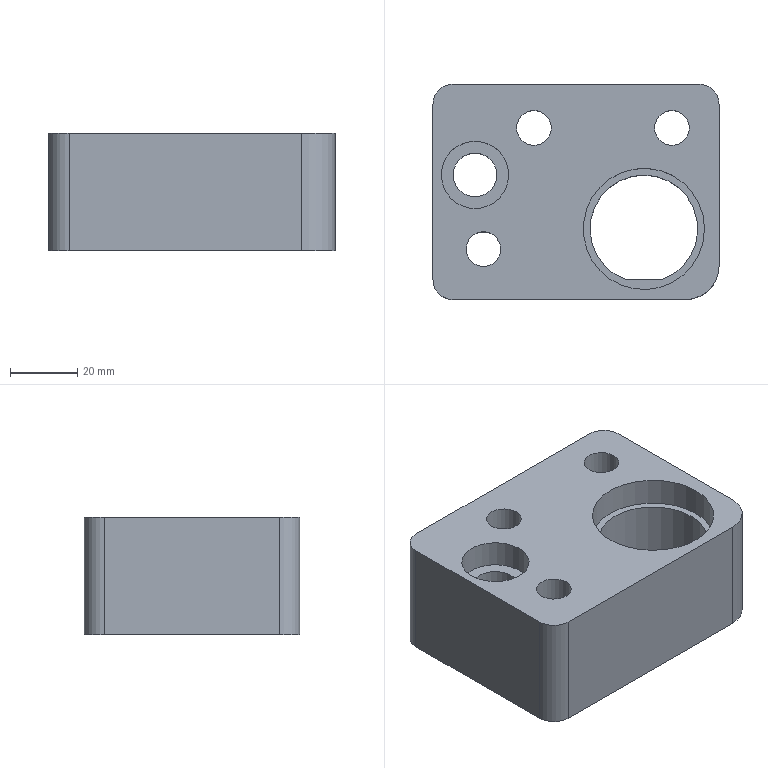Part | NX | features 7 2 | 1 solid | 26 faces | box 85 x 64 x 35 mm | volume 137595 mm3 | cylinder 14 | plane 12 | commonest cylinder face diameters 10.3 x3 12 x3 18 x3 20 x2 13 x1 32 x1
STEP:
#1=CARTESIAN_POINT('',(150.679,-398.,91.));
#2=VERTEX_POINT('',#1);
#3=CARTESIAN_POINT('',(145.529,-398.,91.));
#4=DIRECTION('',(0.,0.,-1.));
#5=DIRECTION('',(1.,0.,0.));
#6=AXIS2_PLACEMENT_3D('',#3,#4,#5);
#7=CIRCLE('',#6,5.15);
#8=EDGE_CURVE('',#2,#2,#7,.T.);
#9=ORIENTED_EDGE('',*,*,#8,.T.);
#10=EDGE_LOOP('',(#9));
#11=FACE_BOUND('',#10,.T.);
#12=CARTESIAN_POINT('',(97.029,-411.95,91.));
#13=VERTEX_POINT('',#12);
#14=CARTESIAN_POINT('',(87.029,-411.95,91.));
#15=DIRECTION('',(0.,0.,-1.));
#16=DIRECTION('',(1.,0.,0.));
#17=AXIS2_PLACEMENT_3D('',#14,#15,#16);
#18=CIRCLE('',#17,10.);
#19=EDGE_CURVE('',#13,#13,#18,.T.);
#20=ORIENTED_EDGE('',*,*,#19,.T.);
#21=EDGE_LOOP('',(#20));
#22=FACE_BOUND('',#21,.T.);
#23=CARTESIAN_POINT('',(155.199,-428.,91.));
#24=VERTEX_POINT('',#23);
#25=CARTESIAN_POINT('',(137.199,-428.,91.));
#26=DIRECTION('',(0.,0.,1.));
#27=DIRECTION('',(1.,0.,0.));
#28=AXIS2_PLACEMENT_3D('',#25,#26,#27);
#29=CIRCLE('',#28,18.);
#30=EDGE_CURVE('',#24,#24,#29,.T.);
#31=ORIENTED_EDGE('',*,*,#30,.F.);
#32=EDGE_LOOP('',(#31));
#33=FACE_BOUND('',#32,.T.);
#34=CARTESIAN_POINT('',(149.529,-449.,91.));
#35=VERTEX_POINT('',#34);
#36=CARTESIAN_POINT('',(80.529,-449.,91.));
#37=VERTEX_POINT('',#36);
#38=CARTESIAN_POINT('',(116.864,-449.,91.));
#39=DIRECTION('',(-1.,0.,0.));
#40=VECTOR('',#39,1000.);
#41=LINE('',#38,#40);
#42=EDGE_CURVE('',#35,#37,#41,.T.);
#43=ORIENTED_EDGE('',*,*,#42,.F.);
#44=CARTESIAN_POINT('',(159.529,-439.,91.));
#45=VERTEX_POINT('',#44);
#46=CARTESIAN_POINT('',(149.529,-439.,91.));
#47=DIRECTION('',(0.,0.,1.));
#48=DIRECTION('',(1.,0.,0.));
#49=AXIS2_PLACEMENT_3D('',#46,#47,#48);
#50=CIRCLE('',#49,10.);
#51=EDGE_CURVE('',#35,#45,#50,.T.);
#52=ORIENTED_EDGE('',*,*,#51,.T.);
#53=CARTESIAN_POINT('',(159.529,-391.,91.));
#54=VERTEX_POINT('',#53);
#55=CARTESIAN_POINT('',(159.529,-424.225,91.));
#56=DIRECTION('',(0.,-1.,0.));
#57=VECTOR('',#56,1000.);
#58=LINE('',#55,#57);
#59=EDGE_CURVE('',#54,#45,#58,.T.);
#60=ORIENTED_EDGE('',*,*,#59,.F.);
#61=CARTESIAN_POINT('',(153.529,-385.,91.));
#62=VERTEX_POINT('',#61);
#63=CARTESIAN_POINT('',(153.529,-391.,91.));
#64=DIRECTION('',(0.,0.,1.));
#65=DIRECTION('',(1.,0.,0.));
#66=AXIS2_PLACEMENT_3D('',#63,#64,#65);
#67=CIRCLE('',#66,6.);
#68=EDGE_CURVE('',#54,#62,#67,.T.);
#69=ORIENTED_EDGE('',*,*,#68,.T.);
#70=CARTESIAN_POINT('',(80.529,-385.,91.));
#71=VERTEX_POINT('',#70);
#72=CARTESIAN_POINT('',(116.864,-385.,91.));
#73=DIRECTION('',(1.,0.,0.));
#74=VECTOR('',#73,1000.);
#75=LINE('',#72,#74);
#76=EDGE_CURVE('',#71,#62,#75,.T.);
#77=ORIENTED_EDGE('',*,*,#76,.F.);
#78=CARTESIAN_POINT('',(74.529,-391.,91.));
#79=VERTEX_POINT('',#78);
#80=CARTESIAN_POINT('',(80.529,-391.,91.));
#81=DIRECTION('',(0.,0.,1.));
#82=DIRECTION('',(1.,0.,0.));
#83=AXIS2_PLACEMENT_3D('',#80,#81,#82);
#84=CIRCLE('',#83,6.);
#85=EDGE_CURVE('',#71,#79,#84,.T.);
#86=ORIENTED_EDGE('',*,*,#85,.T.);
#87=CARTESIAN_POINT('',(74.529,-443.,91.));
#88=VERTEX_POINT('',#87);
#89=CARTESIAN_POINT('',(74.529,-424.225,91.));
#90=DIRECTION('',(0.,1.,0.));
#91=VECTOR('',#90,1000.);
#92=LINE('',#89,#91);
#93=EDGE_CURVE('',#88,#79,#92,.T.);
#94=ORIENTED_EDGE('',*,*,#93,.F.);
#95=CARTESIAN_POINT('',(80.529,-443.,91.));
#96=DIRECTION('',(0.,0.,1.));
#97=DIRECTION('',(1.,0.,0.));
#98=AXIS2_PLACEMENT_3D('',#95,#96,#97);
#99=CIRCLE('',#98,6.);
#100=EDGE_CURVE('',#88,#37,#99,.T.);
#101=ORIENTED_EDGE('',*,*,#100,.T.);
#102=EDGE_LOOP('',(#43,#52,#60,#69,#77,#86,#94,#101));
#103=FACE_BOUND('',#102,.T.);
#104=CARTESIAN_POINT('',(109.679,-398.,91.));
#105=VERTEX_POINT('',#104);
#106=CARTESIAN_POINT('',(104.529,-398.,91.));
#107=DIRECTION('',(0.,0.,-1.));
#108=DIRECTION('',(1.,0.,0.));
#109=AXIS2_PLACEMENT_3D('',#106,#107,#108);
#110=CIRCLE('',#109,5.15);
#111=EDGE_CURVE('',#105,#105,#110,.T.);
#112=ORIENTED_EDGE('',*,*,#111,.T.);
#113=EDGE_LOOP('',(#112));
#114=FACE_BOUND('',#113,.T.);
#115=CARTESIAN_POINT('',(94.679,-434.,91.));
#116=VERTEX_POINT('',#115);
#117=CARTESIAN_POINT('',(89.529,-434.,91.));
#118=DIRECTION('',(0.,0.,-1.));
#119=DIRECTION('',(1.,0.,0.));
#120=AXIS2_PLACEMENT_3D('',#117,#118,#119);
#121=CIRCLE('',#120,5.15);
#122=EDGE_CURVE('',#116,#116,#121,.T.);
#123=ORIENTED_EDGE('',*,*,#122,.T.);
#124=EDGE_LOOP('',(#123));
#125=FACE_BOUND('',#124,.T.);
#126=CARTESIAN_POINT('',(87.029,-411.95,91.));
#127=DIRECTION('',(0.,0.,1.));
#128=DIRECTION('',(-1.,0.,0.));
#129=AXIS2_PLACEMENT_3D('',#126,#127,#128);
#130=PLANE('',#129);
#131=ADVANCED_FACE('',(#11,#22,#33,#103,#114,#125),#130,.T.);
#132=CARTESIAN_POINT('',(154.529,-398.,56.));
#133=VERTEX_POINT('',#132);
#134=CARTESIAN_POINT('',(145.529,-398.,56.));
#135=DIRECTION('',(0.,0.,1.));
#136=DIRECTION('',(1.,0.,0.));
#137=AXIS2_PLACEMENT_3D('',#134,#135,#136);
#138=CIRCLE('',#137,9.);
#139=EDGE_CURVE('',#133,#133,#138,.T.);
#140=ORIENTED_EDGE('',*,*,#139,.T.);
#141=EDGE_LOOP('',(#140));
#142=FACE_BOUND('',#141,.T.);
#143=CARTESIAN_POINT('',(80.529,-411.95,56.));
#144=VERTEX_POINT('',#143);
#145=CARTESIAN_POINT('',(87.029,-411.95,56.));
#146=DIRECTION('',(0.,0.,1.));
#147=DIRECTION('',(-1.,0.,0.));
#148=AXIS2_PLACEMENT_3D('',#145,#146,#147);
#149=CIRCLE('',#148,6.5);
#150=EDGE_CURVE('',#144,#144,#149,.T.);
#151=ORIENTED_EDGE('',*,*,#150,.T.);
#152=EDGE_LOOP('',(#151));
#153=FACE_BOUND('',#152,.T.);
#154=CARTESIAN_POINT('',(142.767,-443.,56.));
#155=VERTEX_POINT('',#154);
#156=CARTESIAN_POINT('',(131.631,-443.,56.));
#157=VERTEX_POINT('',#156);
#158=CARTESIAN_POINT('',(-89.971,-443.,56.));
#159=DIRECTION('',(-1.,0.,0.));
#160=VECTOR('',#159,1000.);
#161=LINE('',#158,#160);
#162=EDGE_CURVE('',#155,#157,#161,.T.);
#163=ORIENTED_EDGE('',*,*,#162,.F.);
#164=CARTESIAN_POINT('',(137.199,-428.,56.));
#165=DIRECTION('',(0.,0.,1.));
#166=DIRECTION('',(-1.,0.,0.));
#167=AXIS2_PLACEMENT_3D('',#164,#165,#166);
#168=CIRCLE('',#167,16.);
#169=EDGE_CURVE('',#155,#157,#168,.T.);
#170=ORIENTED_EDGE('',*,*,#169,.T.);
#171=EDGE_LOOP('',(#163,#170));
#172=FACE_BOUND('',#171,.T.);
#173=CARTESIAN_POINT('',(159.529,-391.,56.));
#174=VERTEX_POINT('',#173);
#175=CARTESIAN_POINT('',(159.529,-439.,56.));
#176=VERTEX_POINT('',#175);
#177=CARTESIAN_POINT('',(159.529,-424.225,56.));
#178=DIRECTION('',(0.,-1.,0.));
#179=VECTOR('',#178,1000.);
#180=LINE('',#177,#179);
#181=EDGE_CURVE('',#174,#176,#180,.T.);
#182=ORIENTED_EDGE('',*,*,#181,.T.);
#183=CARTESIAN_POINT('',(149.529,-449.,56.));
#184=VERTEX_POINT('',#183);
#185=CARTESIAN_POINT('',(149.529,-439.,56.));
#186=DIRECTION('',(0.,0.,-1.));
#187=DIRECTION('',(-1.,0.,0.));
#188=AXIS2_PLACEMENT_3D('',#185,#186,#187);
#189=CIRCLE('',#188,10.);
#190=EDGE_CURVE('',#176,#184,#189,.T.);
#191=ORIENTED_EDGE('',*,*,#190,.T.);
#192=CARTESIAN_POINT('',(80.529,-449.,56.));
#193=VERTEX_POINT('',#192);
#194=CARTESIAN_POINT('',(116.864,-449.,56.));
#195=DIRECTION('',(1.,0.,0.));
#196=VECTOR('',#195,1000.);
#197=LINE('',#194,#196);
#198=EDGE_CURVE('',#193,#184,#197,.T.);
#199=ORIENTED_EDGE('',*,*,#198,.F.);
#200=CARTESIAN_POINT('',(74.529,-443.,56.));
#201=VERTEX_POINT('',#200);
#202=CARTESIAN_POINT('',(80.529,-443.,56.));
#203=DIRECTION('',(0.,0.,-1.));
#204=DIRECTION('',(-1.,0.,0.));
#205=AXIS2_PLACEMENT_3D('',#202,#203,#204);
#206=CIRCLE('',#205,6.);
#207=EDGE_CURVE('',#193,#201,#206,.T.);
#208=ORIENTED_EDGE('',*,*,#207,.T.);
#209=CARTESIAN_POINT('',(74.529,-391.,56.));
#210=VERTEX_POINT('',#209);
#211=CARTESIAN_POINT('',(74.529,-424.225,56.));
#212=DIRECTION('',(0.,-1.,0.));
#213=VECTOR('',#212,1000.);
#214=LINE('',#211,#213);
#215=EDGE_CURVE('',#210,#201,#214,.T.);
#216=ORIENTED_EDGE('',*,*,#215,.F.);
#217=CARTESIAN_POINT('',(80.529,-385.,56.));
#218=VERTEX_POINT('',#217);
#219=CARTESIAN_POINT('',(80.529,-391.,56.));
#220=DIRECTION('',(0.,0.,-1.));
#221=DIRECTION('',(-1.,0.,0.));
#222=AXIS2_PLACEMENT_3D('',#219,#220,#221);
#223=CIRCLE('',#222,6.);
#224=EDGE_CURVE('',#210,#218,#223,.T.);
#225=ORIENTED_EDGE('',*,*,#224,.T.);
#226=CARTESIAN_POINT('',(153.529,-385.,56.));
#227=VERTEX_POINT('',#226);
#228=CARTESIAN_POINT('',(116.864,-385.,56.));
#229=DIRECTION('',(-1.,0.,0.));
#230=VECTOR('',#229,1000.);
#231=LINE('',#228,#230);
#232=EDGE_CURVE('',#227,#218,#231,.T.);
#233=ORIENTED_EDGE('',*,*,#232,.F.);
#234=CARTESIAN_POINT('',(153.529,-391.,56.));
#235=DIRECTION('',(0.,0.,-1.));
#236=DIRECTION('',(-1.,0.,0.));
#237=AXIS2_PLACEMENT_3D('',#234,#235,#236);
#238=CIRCLE('',#237,6.);
#239=EDGE_CURVE('',#227,#174,#238,.T.);
#240=ORIENTED_EDGE('',*,*,#239,.T.);
#241=EDGE_LOOP('',(#182,#191,#199,#208,#216,#225,#233,#240));
#242=FACE_BOUND('',#241,.T.);
#243=CARTESIAN_POINT('',(113.529,-398.,56.));
#244=VERTEX_POINT('',#243);
#245=CARTESIAN_POINT('',(104.529,-398.,56.));
#246=DIRECTION('',(0.,0.,1.));
#247=DIRECTION('',(1.,0.,0.));
#248=AXIS2_PLACEMENT_3D('',#245,#246,#247);
#249=CIRCLE('',#248,9.);
#250=EDGE_CURVE('',#244,#244,#249,.T.);
#251=ORIENTED_EDGE('',*,*,#250,.T.);
#252=EDGE_LOOP('',(#251));
#253=FACE_BOUND('',#252,.T.);
#254=CARTESIAN_POINT('',(98.529,-434.,56.));
#255=VERTEX_POINT('',#254);
#256=CARTESIAN_POINT('',(89.529,-434.,56.));
#257=DIRECTION('',(0.,0.,1.));
#258=DIRECTION('',(1.,0.,0.));
#259=AXIS2_PLACEMENT_3D('',#256,#257,#258);
#260=CIRCLE('',#259,9.);
#261=EDGE_CURVE('',#255,#255,#260,.T.);
#262=ORIENTED_EDGE('',*,*,#261,.T.);
#263=EDGE_LOOP('',(#262));
#264=FACE_BOUND('',#263,.T.);
#265=CARTESIAN_POINT('',(-89.971,-226.95,56.));
#266=DIRECTION('',(0.,0.,-1.));
#267=DIRECTION('',(1.,0.,0.));
#268=AXIS2_PLACEMENT_3D('',#265,#266,#267);
#269=PLANE('',#268);
#270=ADVANCED_FACE('',(#142,#153,#172,#242,#253,#264),#269,.T.);
#271=CARTESIAN_POINT('',(131.631,-443.,82.7));
#272=VERTEX_POINT('',#271);
#273=CARTESIAN_POINT('',(142.767,-443.,82.7));
#274=VERTEX_POINT('',#273);
#275=CARTESIAN_POINT('',(137.199,-443.,82.7));
#276=DIRECTION('',(1.,0.,0.));
#277=VECTOR('',#276,1000.);
#278=LINE('',#275,#277);
#279=EDGE_CURVE('',#272,#274,#278,.T.);
#280=ORIENTED_EDGE('',*,*,#279,.T.);
#281=CARTESIAN_POINT('',(142.767,-443.,121.5));
#282=DIRECTION('',(0.,0.,-1.));
#283=VECTOR('',#282,1000.);
#284=LINE('',#281,#283);
#285=EDGE_CURVE('',#274,#155,#284,.T.);
#286=ORIENTED_EDGE('',*,*,#285,.T.);
#287=ORIENTED_EDGE('',*,*,#162,.T.);
#288=CARTESIAN_POINT('',(131.631,-443.,121.5));
#289=DIRECTION('',(0.,0.,1.));
#290=VECTOR('',#289,1000.);
#291=LINE('',#288,#290);
#292=EDGE_CURVE('',#157,#272,#291,.T.);
#293=ORIENTED_EDGE('',*,*,#292,.T.);
#294=EDGE_LOOP('',(#280,#286,#287,#293));
#295=FACE_BOUND('',#294,.T.);
#296=CARTESIAN_POINT('',(137.199,-443.,83.5));
#297=DIRECTION('',(0.,-1.,0.));
#298=DIRECTION('',(0.,0.,-1.));
#299=AXIS2_PLACEMENT_3D('',#296,#297,#298);
#300=PLANE('',#299);
#301=ADVANCED_FACE('',(#295),#300,.F.);
#302=ORIENTED_EDGE('',*,*,#285,.F.);
#303=CARTESIAN_POINT('',(137.199,-428.,82.7));
#304=DIRECTION('',(0.,0.,-1.));
#305=DIRECTION('',(1.,0.,0.));
#306=AXIS2_PLACEMENT_3D('',#303,#304,#305);
#307=CIRCLE('',#306,16.);
#308=EDGE_CURVE('',#272,#274,#307,.T.);
#309=ORIENTED_EDGE('',*,*,#308,.F.);
#310=ORIENTED_EDGE('',*,*,#292,.F.);
#311=ORIENTED_EDGE('',*,*,#169,.F.);
#312=EDGE_LOOP('',(#302,#309,#310,#311));
#313=FACE_BOUND('',#312,.T.);
#314=CARTESIAN_POINT('',(137.199,-428.,121.5));
#315=DIRECTION('',(0.,0.,-1.));
#316=DIRECTION('',(-1.,0.,0.));
#317=AXIS2_PLACEMENT_3D('',#314,#315,#316);
#318=CYLINDRICAL_SURFACE('',#317,16.);
#319=ADVANCED_FACE('',(#313),#318,.F.);
#320=ORIENTED_EDGE('',*,*,#30,.T.);
#321=EDGE_LOOP('',(#320));
#322=FACE_BOUND('',#321,.T.);
#323=CARTESIAN_POINT('',(155.199,-428.,82.7));
#324=VERTEX_POINT('',#323);
#325=CARTESIAN_POINT('',(137.199,-428.,82.7));
#326=DIRECTION('',(0.,0.,-1.));
#327=DIRECTION('',(1.,0.,0.));
#328=AXIS2_PLACEMENT_3D('',#325,#326,#327);
#329=CIRCLE('',#328,18.);
#330=EDGE_CURVE('',#324,#324,#329,.T.);
#331=ORIENTED_EDGE('',*,*,#330,.T.);
#332=EDGE_LOOP('',(#331));
#333=FACE_BOUND('',#332,.T.);
#334=CARTESIAN_POINT('',(137.199,-428.,91.5));
#335=DIRECTION('',(0.,0.,-1.));
#336=DIRECTION('',(-1.,0.,0.));
#337=AXIS2_PLACEMENT_3D('',#334,#335,#336);
#338=CYLINDRICAL_SURFACE('',#337,18.);
#339=ADVANCED_FACE('',(#322,#333),#338,.F.);
#340=ORIENTED_EDGE('',*,*,#308,.T.);
#341=ORIENTED_EDGE('',*,*,#279,.F.);
#342=EDGE_LOOP('',(#340,#341));
#343=FACE_BOUND('',#342,.T.);
#344=ORIENTED_EDGE('',*,*,#330,.F.);
#345=EDGE_LOOP('',(#344));
#346=FACE_BOUND('',#345,.T.);
#347=CARTESIAN_POINT('',(137.199,-428.,82.7));
#348=DIRECTION('',(0.,0.,1.));
#349=DIRECTION('',(1.,0.,0.));
#350=AXIS2_PLACEMENT_3D('',#347,#348,#349);
#351=PLANE('',#350);
#352=ADVANCED_FACE('',(#343,#346),#351,.T.);
#353=ORIENTED_EDGE('',*,*,#76,.T.);
#354=CARTESIAN_POINT('',(153.529,-385.,19.186));
#355=DIRECTION('',(0.,0.,-1.));
#356=VECTOR('',#355,1000.);
#357=LINE('',#354,#356);
#358=EDGE_CURVE('',#62,#227,#357,.T.);
#359=ORIENTED_EDGE('',*,*,#358,.T.);
#360=ORIENTED_EDGE('',*,*,#232,.T.);
#361=CARTESIAN_POINT('',(80.529,-385.,19.186));
#362=DIRECTION('',(0.,0.,1.));
#363=VECTOR('',#362,1000.);
#364=LINE('',#361,#363);
#365=EDGE_CURVE('',#218,#71,#364,.T.);
#366=ORIENTED_EDGE('',*,*,#365,.T.);
#367=EDGE_LOOP('',(#353,#359,#360,#366));
#368=FACE_BOUND('',#367,.T.);
#369=CARTESIAN_POINT('',(116.864,-385.,19.186));
#370=DIRECTION('',(0.,1.,0.));
#371=DIRECTION('',(0.,0.,-1.));
#372=AXIS2_PLACEMENT_3D('',#369,#370,#371);
#373=PLANE('',#372);
#374=ADVANCED_FACE('',(#368),#373,.T.);
#375=ORIENTED_EDGE('',*,*,#93,.T.);
#376=CARTESIAN_POINT('',(74.529,-391.,19.186));
#377=DIRECTION('',(0.,0.,-1.));
#378=VECTOR('',#377,1000.);
#379=LINE('',#376,#378);
#380=EDGE_CURVE('',#79,#210,#379,.T.);
#381=ORIENTED_EDGE('',*,*,#380,.T.);
#382=ORIENTED_EDGE('',*,*,#215,.T.);
#383=CARTESIAN_POINT('',(74.529,-443.,19.186));
#384=DIRECTION('',(0.,0.,1.));
#385=VECTOR('',#384,1000.);
#386=LINE('',#383,#385);
#387=EDGE_CURVE('',#201,#88,#386,.T.);
#388=ORIENTED_EDGE('',*,*,#387,.T.);
#389=EDGE_LOOP('',(#375,#381,#382,#388));
#390=FACE_BOUND('',#389,.T.);
#391=CARTESIAN_POINT('',(74.529,-424.225,19.186));
#392=DIRECTION('',(-1.,0.,0.));
#393=DIRECTION('',(0.,0.,-1.));
#394=AXIS2_PLACEMENT_3D('',#391,#392,#393);
#395=PLANE('',#394);
#396=ADVANCED_FACE('',(#390),#395,.T.);
#397=ORIENTED_EDGE('',*,*,#198,.T.);
#398=CARTESIAN_POINT('',(149.529,-449.,19.186));
#399=DIRECTION('',(0.,0.,1.));
#400=VECTOR('',#399,1000.);
#401=LINE('',#398,#400);
#402=EDGE_CURVE('',#184,#35,#401,.T.);
#403=ORIENTED_EDGE('',*,*,#402,.T.);
#404=ORIENTED_EDGE('',*,*,#42,.T.);
#405=CARTESIAN_POINT('',(80.529,-449.,19.186));
#406=DIRECTION('',(0.,0.,-1.));
#407=VECTOR('',#406,1000.);
#408=LINE('',#405,#407);
#409=EDGE_CURVE('',#37,#193,#408,.T.);
#410=ORIENTED_EDGE('',*,*,#409,.T.);
#411=EDGE_LOOP('',(#397,#403,#404,#410));
#412=FACE_BOUND('',#411,.T.);
#413=CARTESIAN_POINT('',(116.864,-449.,19.186));
#414=DIRECTION('',(0.,-1.,0.));
#415=DIRECTION('',(0.,0.,1.));
#416=AXIS2_PLACEMENT_3D('',#413,#414,#415);
#417=PLANE('',#416);
#418=ADVANCED_FACE('',(#412),#417,.T.);
#419=ORIENTED_EDGE('',*,*,#59,.T.);
#420=CARTESIAN_POINT('',(159.529,-439.,19.186));
#421=DIRECTION('',(0.,0.,-1.));
#422=VECTOR('',#421,1000.);
#423=LINE('',#420,#422);
#424=EDGE_CURVE('',#45,#176,#423,.T.);
#425=ORIENTED_EDGE('',*,*,#424,.T.);
#426=ORIENTED_EDGE('',*,*,#181,.F.);
#427=CARTESIAN_POINT('',(159.529,-391.,19.186));
#428=DIRECTION('',(0.,0.,1.));
#429=VECTOR('',#428,1000.);
#430=LINE('',#427,#429);
#431=EDGE_CURVE('',#174,#54,#430,.T.);
#432=ORIENTED_EDGE('',*,*,#431,.T.);
#433=EDGE_LOOP('',(#419,#425,#426,#432));
#434=FACE_BOUND('',#433,.T.);
#435=CARTESIAN_POINT('',(159.529,-424.225,19.186));
#436=DIRECTION('',(1.,0.,0.));
#437=DIRECTION('',(0.,0.,1.));
#438=AXIS2_PLACEMENT_3D('',#435,#436,#437);
#439=PLANE('',#438);
#440=ADVANCED_FACE('',(#434),#439,.T.);
#441=CARTESIAN_POINT('',(80.529,-411.95,83.));
#442=VERTEX_POINT('',#441);
#443=CARTESIAN_POINT('',(87.029,-411.95,83.));
#444=DIRECTION('',(0.,0.,-1.));
#445=DIRECTION('',(-1.,0.,0.));
#446=AXIS2_PLACEMENT_3D('',#443,#444,#445);
#447=CIRCLE('',#446,6.5);
#448=EDGE_CURVE('',#442,#442,#447,.T.);
#449=ORIENTED_EDGE('',*,*,#448,.F.);
#450=EDGE_LOOP('',(#449));
#451=FACE_BOUND('',#450,.T.);
#452=ORIENTED_EDGE('',*,*,#150,.F.);
#453=EDGE_LOOP('',(#452));
#454=FACE_BOUND('',#453,.T.);
#455=CARTESIAN_POINT('',(87.029,-411.95,91.));
#456=DIRECTION('',(0.,0.,-1.));
#457=DIRECTION('',(-1.,0.,0.));
#458=AXIS2_PLACEMENT_3D('',#455,#456,#457);
#459=CYLINDRICAL_SURFACE('',#458,6.5);
#460=ADVANCED_FACE('',(#451,#454),#459,.F.);
#461=CARTESIAN_POINT('',(77.029,-411.95,83.));
#462=VERTEX_POINT('',#461);
#463=CARTESIAN_POINT('',(87.029,-411.95,83.));
#464=DIRECTION('',(0.,0.,1.));
#465=DIRECTION('',(-1.,0.,0.));
#466=AXIS2_PLACEMENT_3D('',#463,#464,#465);
#467=CIRCLE('',#466,10.);
#468=EDGE_CURVE('',#462,#462,#467,.T.);
#469=ORIENTED_EDGE('',*,*,#468,.T.);
#470=EDGE_LOOP('',(#469));
#471=FACE_BOUND('',#470,.T.);
#472=ORIENTED_EDGE('',*,*,#448,.T.);
#473=EDGE_LOOP('',(#472));
#474=FACE_BOUND('',#473,.T.);
#475=CARTESIAN_POINT('',(87.029,-411.95,83.));
#476=DIRECTION('',(0.,0.,-1.));
#477=DIRECTION('',(-1.,0.,0.));
#478=AXIS2_PLACEMENT_3D('',#475,#476,#477);
#479=PLANE('',#478);
#480=ADVANCED_FACE('',(#471,#474),#479,.F.);
#481=ORIENTED_EDGE('',*,*,#19,.F.);
#482=EDGE_LOOP('',(#481));
#483=FACE_BOUND('',#482,.T.);
#484=ORIENTED_EDGE('',*,*,#468,.F.);
#485=EDGE_LOOP('',(#484));
#486=FACE_BOUND('',#485,.T.);
#487=CARTESIAN_POINT('',(87.029,-411.95,90.559));
#488=DIRECTION('',(0.,0.,-1.));
#489=DIRECTION('',(1.,0.,0.));
#490=AXIS2_PLACEMENT_3D('',#487,#488,#489);
#491=CYLINDRICAL_SURFACE('',#490,10.);
#492=ADVANCED_FACE('',(#483,#486),#491,.F.);
#493=ORIENTED_EDGE('',*,*,#190,.F.);
#494=ORIENTED_EDGE('',*,*,#424,.F.);
#495=ORIENTED_EDGE('',*,*,#51,.F.);
#496=ORIENTED_EDGE('',*,*,#402,.F.);
#497=EDGE_LOOP('',(#493,#494,#495,#496));
#498=FACE_BOUND('',#497,.T.);
#499=CARTESIAN_POINT('',(149.529,-439.,19.186));
#500=DIRECTION('',(0.,0.,-1.));
#501=DIRECTION('',(1.,0.,0.));
#502=AXIS2_PLACEMENT_3D('',#499,#500,#501);
#503=CYLINDRICAL_SURFACE('',#502,10.);
#504=ADVANCED_FACE('',(#498),#503,.T.);
#505=ORIENTED_EDGE('',*,*,#239,.F.);
#506=ORIENTED_EDGE('',*,*,#358,.F.);
#507=ORIENTED_EDGE('',*,*,#68,.F.);
#508=ORIENTED_EDGE('',*,*,#431,.F.);
#509=EDGE_LOOP('',(#505,#506,#507,#508));
#510=FACE_BOUND('',#509,.T.);
#511=CARTESIAN_POINT('',(153.529,-391.,19.186));
#512=DIRECTION('',(0.,0.,1.));
#513=DIRECTION('',(-1.,0.,0.));
#514=AXIS2_PLACEMENT_3D('',#511,#512,#513);
#515=CYLINDRICAL_SURFACE('',#514,6.);
#516=ADVANCED_FACE('',(#510),#515,.T.);
#517=ORIENTED_EDGE('',*,*,#224,.F.);
#518=ORIENTED_EDGE('',*,*,#380,.F.);
#519=ORIENTED_EDGE('',*,*,#85,.F.);
#520=ORIENTED_EDGE('',*,*,#365,.F.);
#521=EDGE_LOOP('',(#517,#518,#519,#520));
#522=FACE_BOUND('',#521,.T.);
#523=CARTESIAN_POINT('',(80.529,-391.,19.186));
#524=DIRECTION('',(0.,0.,1.));
#525=DIRECTION('',(-1.,0.,0.));
#526=AXIS2_PLACEMENT_3D('',#523,#524,#525);
#527=CYLINDRICAL_SURFACE('',#526,6.);
#528=ADVANCED_FACE('',(#522),#527,.T.);
#529=ORIENTED_EDGE('',*,*,#207,.F.);
#530=ORIENTED_EDGE('',*,*,#409,.F.);
#531=ORIENTED_EDGE('',*,*,#100,.F.);
#532=ORIENTED_EDGE('',*,*,#387,.F.);
#533=EDGE_LOOP('',(#529,#530,#531,#532));
#534=FACE_BOUND('',#533,.T.);
#535=CARTESIAN_POINT('',(80.529,-443.,19.186));
#536=DIRECTION('',(0.,0.,1.));
#537=DIRECTION('',(-1.,0.,0.));
#538=AXIS2_PLACEMENT_3D('',#535,#536,#537);
#539=CYLINDRICAL_SURFACE('',#538,6.);
#540=ADVANCED_FACE('',(#534),#539,.T.);
#541=CARTESIAN_POINT('',(109.679,-398.,69.));
#542=VERTEX_POINT('',#541);
#543=CARTESIAN_POINT('',(104.529,-398.,69.));
#544=DIRECTION('',(0.,0.,1.));
#545=DIRECTION('',(1.,0.,0.));
#546=AXIS2_PLACEMENT_3D('',#543,#544,#545);
#547=CIRCLE('',#546,5.15);
#548=EDGE_CURVE('',#542,#542,#547,.T.);
#549=ORIENTED_EDGE('',*,*,#548,.F.);
#550=EDGE_LOOP('',(#549));
#551=FACE_BOUND('',#550,.T.);
#552=ORIENTED_EDGE('',*,*,#111,.F.);
#553=EDGE_LOOP('',(#552));
#554=FACE_BOUND('',#553,.T.);
#555=CARTESIAN_POINT('',(104.529,-398.,56.));
#556=DIRECTION('',(0.,0.,1.));
#557=DIRECTION('',(-1.,0.,0.));
#558=AXIS2_PLACEMENT_3D('',#555,#556,#557);
#559=CYLINDRICAL_SURFACE('',#558,5.15);
#560=ADVANCED_FACE('',(#551,#554),#559,.F.);
#561=ORIENTED_EDGE('',*,*,#548,.T.);
#562=EDGE_LOOP('',(#561));
#563=FACE_BOUND('',#562,.T.);
#564=CARTESIAN_POINT('',(113.529,-398.,69.));
#565=VERTEX_POINT('',#564);
#566=CARTESIAN_POINT('',(104.529,-398.,69.));
#567=DIRECTION('',(0.,0.,1.));
#568=DIRECTION('',(1.,0.,0.));
#569=AXIS2_PLACEMENT_3D('',#566,#567,#568);
#570=CIRCLE('',#569,9.);
#571=EDGE_CURVE('',#565,#565,#570,.T.);
#572=ORIENTED_EDGE('',*,*,#571,.F.);
#573=EDGE_LOOP('',(#572));
#574=FACE_BOUND('',#573,.T.);
#575=CARTESIAN_POINT('',(104.529,-398.,69.));
#576=DIRECTION('',(0.,0.,1.));
#577=DIRECTION('',(-1.,0.,0.));
#578=AXIS2_PLACEMENT_3D('',#575,#576,#577);
#579=PLANE('',#578);
#580=ADVANCED_FACE('',(#563,#574),#579,.F.);
#581=ORIENTED_EDGE('',*,*,#571,.T.);
#582=EDGE_LOOP('',(#581));
#583=FACE_BOUND('',#582,.T.);
#584=ORIENTED_EDGE('',*,*,#250,.F.);
#585=EDGE_LOOP('',(#584));
#586=FACE_BOUND('',#585,.T.);
#587=CARTESIAN_POINT('',(104.529,-398.,56.));
#588=DIRECTION('',(0.,0.,1.));
#589=DIRECTION('',(-1.,0.,0.));
#590=AXIS2_PLACEMENT_3D('',#587,#588,#589);
#591=CYLINDRICAL_SURFACE('',#590,9.);
#592=ADVANCED_FACE('',(#583,#586),#591,.F.);
#593=CARTESIAN_POINT('',(150.679,-398.,69.));
#594=VERTEX_POINT('',#593);
#595=CARTESIAN_POINT('',(145.529,-398.,69.));
#596=DIRECTION('',(0.,0.,1.));
#597=DIRECTION('',(1.,0.,0.));
#598=AXIS2_PLACEMENT_3D('',#595,#596,#597);
#599=CIRCLE('',#598,5.15);
#600=EDGE_CURVE('',#594,#594,#599,.T.);
#601=ORIENTED_EDGE('',*,*,#600,.F.);
#602=EDGE_LOOP('',(#601));
#603=FACE_BOUND('',#602,.T.);
#604=ORIENTED_EDGE('',*,*,#8,.F.);
#605=EDGE_LOOP('',(#604));
#606=FACE_BOUND('',#605,.T.);
#607=CARTESIAN_POINT('',(145.529,-398.,56.));
#608=DIRECTION('',(0.,0.,1.));
#609=DIRECTION('',(-1.,0.,0.));
#610=AXIS2_PLACEMENT_3D('',#607,#608,#609);
#611=CYLINDRICAL_SURFACE('',#610,5.15);
#612=ADVANCED_FACE('',(#603,#606),#611,.F.);
#613=ORIENTED_EDGE('',*,*,#600,.T.);
#614=EDGE_LOOP('',(#613));
#615=FACE_BOUND('',#614,.T.);
#616=CARTESIAN_POINT('',(154.529,-398.,69.));
#617=VERTEX_POINT('',#616);
#618=CARTESIAN_POINT('',(145.529,-398.,69.));
#619=DIRECTION('',(0.,0.,1.));
#620=DIRECTION('',(1.,0.,0.));
#621=AXIS2_PLACEMENT_3D('',#618,#619,#620);
#622=CIRCLE('',#621,9.);
#623=EDGE_CURVE('',#617,#617,#622,.T.);
#624=ORIENTED_EDGE('',*,*,#623,.F.);
#625=EDGE_LOOP('',(#624));
#626=FACE_BOUND('',#625,.T.);
#627=CARTESIAN_POINT('',(145.529,-398.,69.));
#628=DIRECTION('',(0.,0.,1.));
#629=DIRECTION('',(-1.,0.,0.));
#630=AXIS2_PLACEMENT_3D('',#627,#628,#629);
#631=PLANE('',#630);
#632=ADVANCED_FACE('',(#615,#626),#631,.F.);
#633=ORIENTED_EDGE('',*,*,#623,.T.);
#634=EDGE_LOOP('',(#633));
#635=FACE_BOUND('',#634,.T.);
#636=ORIENTED_EDGE('',*,*,#139,.F.);
#637=EDGE_LOOP('',(#636));
#638=FACE_BOUND('',#637,.T.);
#639=CARTESIAN_POINT('',(145.529,-398.,56.));
#640=DIRECTION('',(0.,0.,1.));
#641=DIRECTION('',(-1.,0.,0.));
#642=AXIS2_PLACEMENT_3D('',#639,#640,#641);
#643=CYLINDRICAL_SURFACE('',#642,9.);
#644=ADVANCED_FACE('',(#635,#638),#643,.F.);
#645=CARTESIAN_POINT('',(94.679,-434.,69.));
#646=VERTEX_POINT('',#645);
#647=CARTESIAN_POINT('',(89.529,-434.,69.));
#648=DIRECTION('',(0.,0.,1.));
#649=DIRECTION('',(1.,0.,0.));
#650=AXIS2_PLACEMENT_3D('',#647,#648,#649);
#651=CIRCLE('',#650,5.15);
#652=EDGE_CURVE('',#646,#646,#651,.T.);
#653=ORIENTED_EDGE('',*,*,#652,.F.);
#654=EDGE_LOOP('',(#653));
#655=FACE_BOUND('',#654,.T.);
#656=ORIENTED_EDGE('',*,*,#122,.F.);
#657=EDGE_LOOP('',(#656));
#658=FACE_BOUND('',#657,.T.);
#659=CARTESIAN_POINT('',(89.529,-434.,56.));
#660=DIRECTION('',(0.,0.,1.));
#661=DIRECTION('',(-1.,0.,0.));
#662=AXIS2_PLACEMENT_3D('',#659,#660,#661);
#663=CYLINDRICAL_SURFACE('',#662,5.15);
#664=ADVANCED_FACE('',(#655,#658),#663,.F.);
#665=ORIENTED_EDGE('',*,*,#652,.T.);
#666=EDGE_LOOP('',(#665));
#667=FACE_BOUND('',#666,.T.);
#668=CARTESIAN_POINT('',(98.529,-434.,69.));
#669=VERTEX_POINT('',#668);
#670=CARTESIAN_POINT('',(89.529,-434.,69.));
#671=DIRECTION('',(0.,0.,1.));
#672=DIRECTION('',(1.,0.,0.));
#673=AXIS2_PLACEMENT_3D('',#670,#671,#672);
#674=CIRCLE('',#673,9.);
#675=EDGE_CURVE('',#669,#669,#674,.T.);
#676=ORIENTED_EDGE('',*,*,#675,.F.);
#677=EDGE_LOOP('',(#676));
#678=FACE_BOUND('',#677,.T.);
#679=CARTESIAN_POINT('',(89.529,-434.,69.));
#680=DIRECTION('',(0.,0.,1.));
#681=DIRECTION('',(-1.,0.,0.));
#682=AXIS2_PLACEMENT_3D('',#679,#680,#681);
#683=PLANE('',#682);
#684=ADVANCED_FACE('',(#667,#678),#683,.F.);
#685=ORIENTED_EDGE('',*,*,#675,.T.);
#686=EDGE_LOOP('',(#685));
#687=FACE_BOUND('',#686,.T.);
#688=ORIENTED_EDGE('',*,*,#261,.F.);
#689=EDGE_LOOP('',(#688));
#690=FACE_BOUND('',#689,.T.);
#691=CARTESIAN_POINT('',(89.529,-434.,56.));
#692=DIRECTION('',(0.,0.,1.));
#693=DIRECTION('',(-1.,0.,0.));
#694=AXIS2_PLACEMENT_3D('',#691,#692,#693);
#695=CYLINDRICAL_SURFACE('',#694,9.);
#696=ADVANCED_FACE('',(#687,#690),#695,.F.);
#697=CLOSED_SHELL('',(#131,#270,#301,#319,#339,#352,#374,#396,#418,#440,#460,#480,#492,#504,#516,#528,#540,#560,#580,#592,#612,#632,#644,#664,#684,#696));
#698=MANIFOLD_SOLID_BREP('',#697);
#699=(LENGTH_UNIT()NAMED_UNIT(*)SI_UNIT(.MILLI.,.METRE.));
#700=UNCERTAINTY_MEASURE_WITH_UNIT(LENGTH_MEASURE(0.00001),#699,'','');
#701=(NAMED_UNIT(*)PLANE_ANGLE_UNIT()SI_UNIT($,.RADIAN.));
#702=(NAMED_UNIT(*)SI_UNIT($,.STERADIAN.)SOLID_ANGLE_UNIT());
#703=(GEOMETRIC_REPRESENTATION_CONTEXT(3)GLOBAL_UNCERTAINTY_ASSIGNED_CONTEXT((#700))GLOBAL_UNIT_ASSIGNED_CONTEXT((#699,#701,#702))REPRESENTATION_CONTEXT('',''));
#704=ADVANCED_BREP_SHAPE_REPRESENTATION('',(#698),#703);